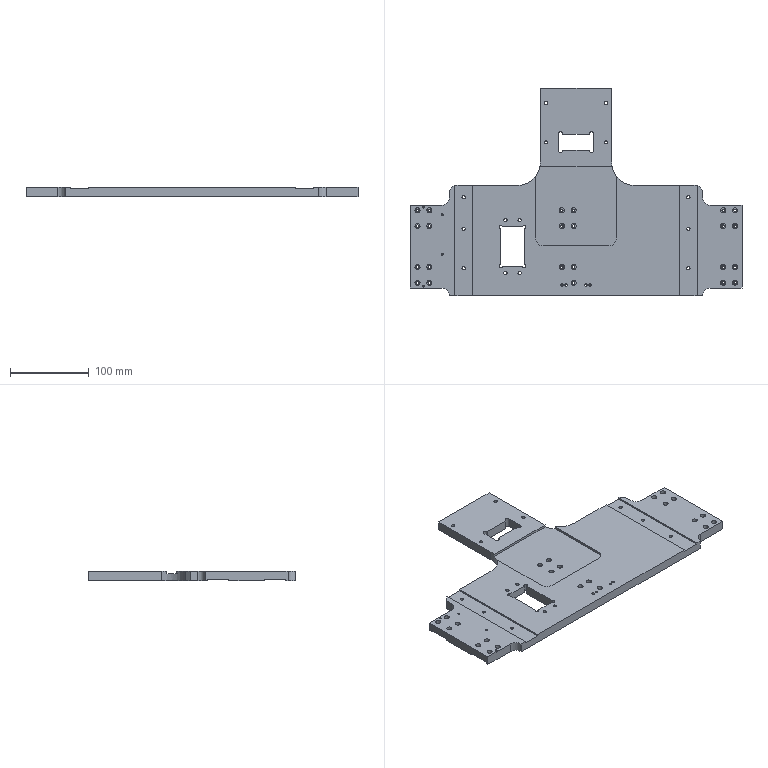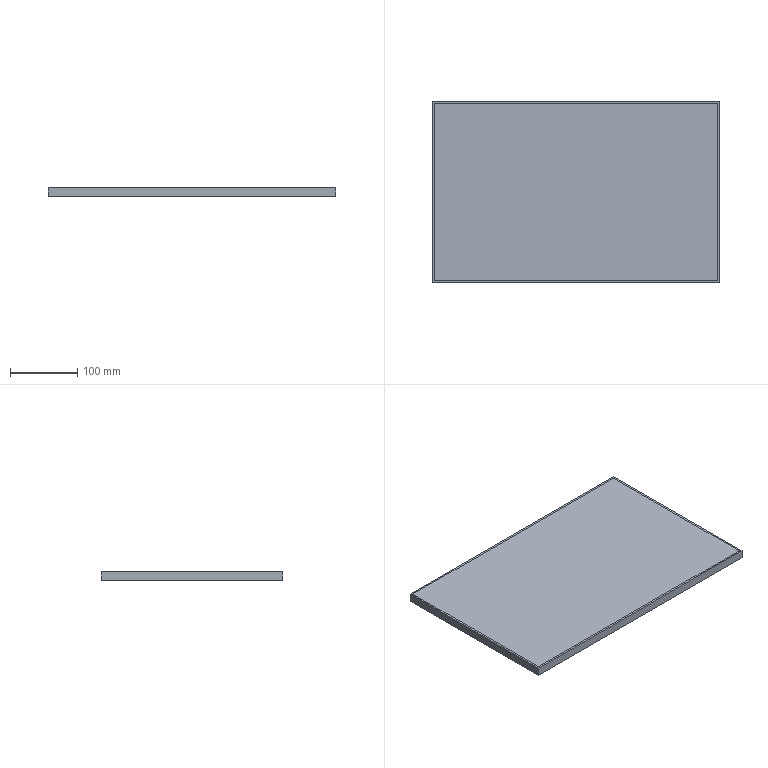CAM job | NX | 3-axis milling, drilling | part box 421 x 263.5 x 12 mm | stock box 427 x 269.5 x 13 mm
Tools:
number,name,description,diameter,corner_radius,flute_length,length,flutes
10,D10,Milling Tool-5 Parameters,10.0,0.0,50.0,75.0,2
1,D63,Milling Tool-5 Parameters,63.0,0.0,50.0,75.0,2
7,D6A45,Milling Tool-5 Parameters,6.0,0.0,3.0,3.0,2
13,3.4ZT,Drilling Tool,3.3,0.0,35.0,50.0,2
17,M4,Milling Tool-5 Parameters,3.3,0.0,30.0,30.0,4
8,2.5ZT,Drilling Tool,2.5,0.0,35.0,50.0,2
9,M3,Milling Tool-5 Parameters,2.5,0.0,30.0,30.0,4
14,4.2ZT,Drilling Tool,4.2,0.0,35.0,50.0,2
15,M5,Milling Tool-5 Parameters,4.2,0.0,30.0,30.0,4
18,2.8ZT,Drilling Tool,2.8,0.0,35.0,50.0,2
19,3.0JD,Milling Tool-5 Parameters,3.0,0.0,30.0,30.0,4
11,D10JING,Milling Tool-5 Parameters,10.0,0.0,50.0,75.0,2
4,D4,Milling Tool-5 Parameters,4.0,0.0,50.0,75.0,2
Operations:
program,operation,operation_type,tool,method,geometry_group,spindle_rpm,surface_speed,feed_per_tooth,feed_cut,feed_plunge,cut_length_mm,path_length_mm,cut_time_min,machine_time_min
1-424-268-12-AB胶,FLOOR_WALL,VolumeBased25DMillingOperation,D63,METHOD,A,6500.0,1286.0,0.0962,1250.0,100.0,4666.297,4720.297,3.733,3.738
1-424-268-12-AB胶,DRILLING_COPY_1,Operation,D6A45,METHOD,A,3000.0,56.0,0.0333,200.0,0.0,212.0,2091.358,1.06,1.248
1-424-268-12-AB胶,DRILLING_COPY_1_COPY_COPY_COPY_COPY_COPY,Operation,3.4ZT,METHOD,A,2000.0,20.0,0.0375,150.0,0.0,333.303,1596.175,2.222,2.348
1-424-268-12-AB胶,DRILLING_COPY_1_COPY_COPY_COPY_COPY_COPY_COPY_1,Operation,3.4ZT,METHOD,A,2000.0,20.0,0.0375,150.0,0.0,27.342,153.808,0.1823,0.1949
1-424-268-12-AB胶,DRILLING_COPY_1_COPY_COPY_COPY_COPY_COPY_COPY,Operation,M4,METHOD,A,200.0,2.0,0.175,140.0,0.0,20.0,139.125,0.1429,0.1548
1-424-268-12-AB胶,DRILLING_COPY_1_COPY_1,Operation,2.5ZT,METHOD,A,2000.0,15.0,0.0375,150.0,0.0,45.004,282.113,0.3,0.3237
1-424-268-12-AB胶,DRILLING_COPY_1_COPY_COPY_2,Operation,M3,METHOD,A,200.0,1.0,0.125,100.0,0.0,42.0,329.028,0.42,0.4487
1-424-268-12-AB胶,DRILLING_COPY_1_COPY,Operation,4.2ZT,METHOD,A,2000.0,15.0,0.0375,150.0,0.0,236.665,1309.304,1.578,1.685
1-424-268-12-AB胶,DRILLING_COPY_1_COPY_COPY_3,Operation,4.2ZT,METHOD,A,2000.0,15.0,0.0375,150.0,0.0,67.047,313.484,0.447,0.4716
1-424-268-12-AB胶,DRILLING_COPY_1_COPY_COPY_3_COPY,Operation,4.2ZT,METHOD,A,2000.0,15.0,0.0375,150.0,0.0,67.047,301.895,0.447,0.4705
1-424-268-12-AB胶,DRILLING_COPY_1_COPY_COPY,Operation,M5,METHOD,A,200.0,2.0,0.2,160.0,0.0,205.0,1245.974,1.281,1.385
1-424-268-12-AB胶,DRILLING_COPY_1_COPY_COPY_1,Operation,2.8ZT,METHOD,A,2000.0,15.0,0.0375,150.0,0.0,34.682,157.544,0.2312,0.2435
1-424-268-12-AB胶,DRILLING_COPY_1_COPY_COPY_1_COPY,Operation,3.0JD,METHOD,A,1000.0,9.0,0.0125,50.0,0.0,31.0,150.179,0.62,0.6319
1-424-268-12-AB胶,ZLEVEL_PROFILE,ZLevelMilling,D10,METHOD,A,7000.0,219.0,0.2143,3000.0,1000.0,16315.963,16384.363,5.47,5.477
1-424-268-12-AB胶,CAVITY_MILL,CavityMilling,D10,METHOD,A,7000.0,439.0,0.1571,2200.0,1000.0,7666.404,8656.634,4.298,4.438
1-424-268-12-AB胶,11,VolumeBased25DMillingOperation,D10,METHOD,A,7000.0,219.0,0.1429,2000.0,100.0,11205.802,12352.694,5.603,5.723
1-424-268-12-AB胶,FLOOR_WALL_1_COPY_1,VolumeBased25DMillingOperation,D10JING,METHOD,A,7000.0,87.0,0.0714,1000.0,100.0,4140.319,5004.687,4.14,4.227
1-424-268-12-AB胶,HOLE_MILLING,CylinderMilling,D4,METHOD,A,7000.0,131.0,0.0714,1000.0,100.0,4114.36,6454.017,4.114,4.348
1-424-268-12-AB胶,ZLEVEL_PROFILE_COPY_1,ZLevelMilling,D4,METHOD,A,7000.0,87.0,0.1071,1500.0,1000.0,2630.535,4605.289,1.842,2.039
1-424-268-12-AB胶,ZLEVEL_PROFILE_COPY_1_COPY_COPY_COPY_COPY_2_COPY,ZLevelMilling,D6A45,METHOD,A,7000.0,131.0,0.0714,1000.0,1000.0,2921.034,7890.41,2.921,3.418
1-424-268-12-AB胶,ZLEVEL_PROFILE_COPY_1_COPY_COPY_COPY_COPY_2_COPY_COPY,ZLevelMilling,D6A45,METHOD,A,7000.0,131.0,0.0714,1000.0,1000.0,127.352,3058.598,0.1274,0.4205
1-424-268-12-AB胶,ZLEVEL_PROFILE_COPY_1_COPY_COPY_COPY_COPY_2_COPY_COPY_COPY,ZLevelMilling,D6A45,METHOD,A,7000.0,131.0,0.0714,1000.0,1000.0,71.875,742.825,0.0719,0.139
1-424-268-12-AB胶,刀补11,VolumeBased25DMillingOperation,D10JING,METHOD,A,7000.0,87.0,0.0714,1000.0,100.0,1053.055,1633.176,1.053,1.111
1-424-268-12-AB胶,刀补4,ZLevelMilling,D4,METHOD,A,7000.0,87.0,0.0607,850.0,1000.0,557.813,893.918,0.6556,0.6892
1-424-268-12-AB胶,ZLEVEL_PROFILE_COPY_1_1,ZLevelMilling,D10JING,METHOD,A,7000.0,219.0,0.0714,1000.0,1000.0,4284.642,4355.392,4.285,4.292
2-424-268-12-AB胶,FLOOR_WALL_COPY,VolumeBased25DMillingOperation,D63,METHOD,B,6500.0,1286.0,0.0962,1250.0,100.0,3424.223,3478.223,2.739,2.745
2-424-268-12-AB胶,1212,VolumeBased25DMillingOperation,D10,METHOD,B,7000.0,219.0,0.1429,2000.0,100.0,10495.664,10743.709,5.248,5.275
2-424-268-12-AB胶,FLOOR_WALL_1_COPY_1_COPY,VolumeBased25DMillingOperation,D10JING,METHOD,B,7000.0,87.0,0.0714,1000.0,100.0,6113.68,6744.276,6.114,6.18
2-424-268-12-AB胶,ZLEVEL_PROFILE_COPY_1_COPY_COPY_COPY_COPY_2_COPY_COPY_1,ZLevelMilling,D6A45,METHOD,B,7000.0,131.0,0.0714,1000.0,1000.0,3161.762,5183.983,3.162,3.364
2-424-268-12-AB胶,ZLEVEL_PROFILE_COPY_1_COPY_COPY_COPY_COPY_2_COPY_COPY_1_COPY,ZLevelMilling,D6A45,METHOD,B,7000.0,131.0,0.0714,1000.0,1000.0,307.46,7818.298,0.3075,1.058
2-424-268-12-AB胶,刀补11_COPY,VolumeBased25DMillingOperation,D10JING,METHOD,B,7000.0,87.0,0.0714,1000.0,100.0,1754.87,1996.406,1.755,1.781